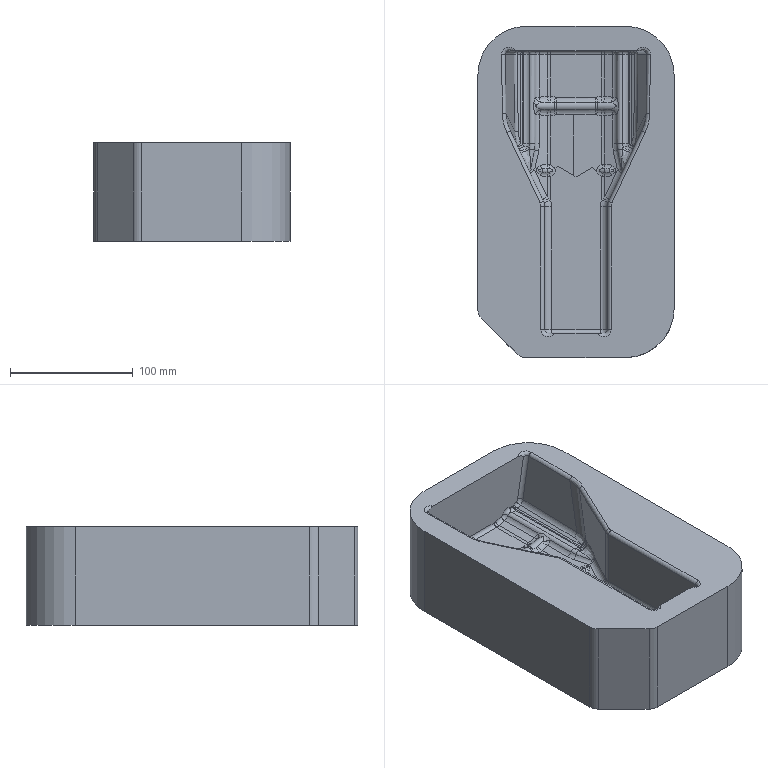NC program | NX | posted with a generic post | part box 160 x 270 x 80 mm
Lines 11488 to 12477 of 159324:
(ZLEVEL_PROFILE , TOOL : D16R0.8)
N22974 M6
N22976 G54
N22978 G17 G0 G90 X-41.264 Y99.089 S2000 M3
N22980 G43 Z10. H0
N22982 Z2.801
N22984 G94 G1 Z-0.199 F2000.
N22986 G3 X-49.234 Y107.089 R8.
N22988 G2 X-51.725 Y107.343 R12.794
N22990 G1 X-51.154 Y64.218
N22992 G3 X-48.351 Y52.165 R29.228
N22994 G1 X-21.353 Y-5.208
N22996 G2 X-19.849 Y-11.942 R15.824
N22998 G1 Y-107.329
N23000 G2 X-17.058 Y-107.089 R12.418
N23002 G1 X-17.202 Y-106.964 Z-0.399
N23004 G3 X-19.464 Y-107.098 R15.796
N23006 G1 Y-11.942
N23008 G3 X-21.005 Y-5.045 R16.209
N23010 G1 X-48.003 Y52.329
N23012 G2 X-50.77 Y64.256 R28.919
N23014 G1 X-51.337 Y107.111
N23016 G3 X-49.234 Y106.964 R14.071
N23018 G1 X-49.605 Y106.897 Z-0.598
N23020 X-51.031 Y106.963
N23022 X-50.465 Y64.227
N23024 G3 X-47.701 Y52.404 R28.679
N23026 G1 X-20.735 Y-4.902
N23028 G2 X-19.16 Y-11.942 R16.513
N23030 G1 Y-106.97
N23032 X-17.59 Y-106.898
N23034 X-17.299 Y-106.897
N23036 X-17.569 Y-106.885 Z-0.698
N23038 X-17.84 Y-106.875 Z-0.798
N23040 X-18.906 Y-106.886
N23042 Y-11.942
N23044 G3 X-20.498 Y-4.811 R16.767
N23046 G1 X-47.465 Y52.498
N23048 G2 X-50.213 Y64.315 R28.655
N23050 G1 X-50.776 Y106.897
N23052 X-49.917 Y106.875
N23054 G2 X-42.126 Y98.875 R8.
N23056 G1 Z2.202
N23058 G0 Z10.
N23060 X8.831 Y-99.089
N23062 Z2.801
N23064 G1 Z-0.199
N23066 X8.838 Y-99.326
N23068 G3 X17.068 Y-107.089 R8.
N23070 G2 X19.849 Y-107.333 R11.98
N23072 G1 Y-11.942
N23074 G2 X21.355 Y-5.203 R15.824
N23076 G1 X48.351 Y52.165
N23078 G3 X51.154 Y64.218 R29.228
N23080 G1 X51.725 Y107.339
N23082 G2 X49.244 Y107.089 R12.65
N23084 G1 Y107.018 Z-0.299
N23086 Y106.964 Z-0.399
N23088 G3 X51.337 Y107.111 R14.232
N23090 G1 X50.77 Y64.223
N23092 G2 X48.003 Y52.329 R28.844
N23094 G1 X21.005 Y-5.044
N23096 G3 X19.464 Y-11.942 R16.209
N23098 G1 Y-107.095
N23100 G3 X17.361 Y-106.964 R16.476
N23102 G1 X17.647 Y-106.897 Z-0.598
N23104 X19.16 Y-106.962
N23106 Y-11.942
N23108 G2 X20.735 Y-4.902 R16.513
N23110 G1 X47.704 Y52.41
N23112 G3 X50.465 Y64.227 R28.664
N23114 G1 X51.031 Y106.97
N23116 X49.401 Y106.898
N23118 X49.244 Y106.897
N23120 X49.581 Y106.888 Z-0.698
N23122 X49.919 Y106.875 Z-0.798
N23124 X50.776 Y106.898
N23126 X50.213 Y64.327
N23128 G2 X47.469 Y52.507 R28.661
N23130 G1 X20.504 Y-4.799
N23132 G3 X18.906 Y-11.942 R16.767
N23134 G1 Y-106.889
N23136 X17.836 Y-106.875
N23138 G2 X9.938 Y-98.875 R8.
N23140 G1 Z2.202
N23142 G0 Z10.
N23144 X8. Y98.875
N23146 Z2.003
N23148 G1 Z-0.997
N23150 G3 X0. Y106.875 R8.
N23152 G1 X-50.559
N23154 X-49.996 Y64.264
N23156 G3 X-47.339 Y52.738 R27.939
N23158 G1 X-20.298 Y-4.729
N23160 G2 X-18.69 Y-11.942 R16.983
N23162 G1 Y-106.875
N23164 X18.69
N23166 Y-11.942
N23168 G2 X20.308 Y-4.707 R16.983
N23170 G1 X47.282 Y52.617
N23172 G3 X49.995 Y64.233 R28.176
N23174 G1 X50.559 Y106.875
N23176 X0.
N23178 Z-1.197
N23180 X50.372
N23182 X49.808 Y64.236
N23184 G2 X47.115 Y52.701 R27.978
N23186 G1 X20.138 Y-4.627
N23188 G3 X18.502 Y-11.942 R17.171
N23190 G1 Y-106.875
N23192 X-18.502
N23194 Y-11.942
N23196 G3 X-20.128 Y-4.649 R17.171
N23198 G1 X-47.132 Y52.739
N23200 G2 X-49.808 Y64.236 R27.882
N23202 G1 X-50.372 Y106.875
N23204 X0.
N23206 Z-1.396
N23208 X-50.208
N23210 X-49.645 Y64.242
N23212 G3 X-46.984 Y52.808 R27.729
N23214 G1 X-19.988 Y-4.563
N23216 G2 X-18.339 Y-11.942 R17.334
N23218 G1 Y-106.875
N23220 X18.339
N23222 Y-11.942
N23224 G2 X19.989 Y-4.559 R17.334
N23226 G1 X46.969 Y52.775
N23228 G3 X49.645 Y64.272 R27.397
N23230 G1 X50.208 Y106.875
N23232 X0.
N23234 Z-1.596
N23236 X50.065
N23238 X49.501 Y64.24
N23240 G2 X46.84 Y52.839 R27.11
N23242 G1 X19.862 Y-4.493
N23244 G3 X18.195 Y-11.942 R17.478
N23246 G1 Y-106.875
N23248 X-18.195
N23250 Y-11.942
N23252 G3 X-19.855 Y-4.508 R17.478
N23254 G1 X-46.84 Y52.838
N23256 G2 X-49.501 Y64.24 R27.655
N23258 G1 X-50.065 Y106.875
N23260 X0.
N23262 Z-1.795
N23264 X-49.939
N23266 X-49.376 Y64.283
N23268 G3 X-46.741 Y52.923 R27.331
N23270 G1 X-19.741 Y-4.456
N23272 G2 X-18.07 Y-11.942 R17.603
N23274 G1 Y-106.875
N23276 X18.07
N23278 Y-11.942
N23280 G2 X19.748 Y-4.441 R17.603
N23282 G1 X46.741 Y52.923
N23284 G3 X49.375 Y64.242 R27.192
N23286 G1 X49.939 Y106.875
N23288 X0.
N23290 Z-1.995
N23292 X49.829
N23294 X49.267 Y64.327
N23296 G2 X46.633 Y52.952 R27.37
N23298 G1 X19.648 Y-4.395
N23300 G3 X17.96 Y-11.942 R17.713
N23302 G1 Y-106.875
N23304 X-17.96
N23306 Y-11.942
N23308 G3 X-19.641 Y-4.41 R17.713
N23310 G1 X-46.629 Y52.942
N23312 G2 X-49.266 Y64.304 R27.361
N23314 G1 X-49.829 Y106.875
N23316 X0.
N23318 Z-2.194
N23320 X-49.734
N23322 X-49.17 Y64.244
N23324 G3 X-46.555 Y53.01 R27.444
N23326 G1 X-19.554 Y-4.37
N23328 G2 X-17.864 Y-11.942 R17.809
N23330 G1 Y-106.875
N23332 X17.864
N23334 Y-11.942
N23336 G2 X19.561 Y-4.355 R17.809
N23338 G1 X46.555 Y53.01
N23340 G3 X49.17 Y64.251 R27.431
N23342 G1 X49.734 Y106.875
N23344 X0.
N23346 Z-2.393
N23348 X49.652
N23350 X49.088 Y64.245
N23352 G2 X46.465 Y53.013 R27.246
N23354 G1 X19.486 Y-4.321
N23356 G3 X17.782 Y-11.942 R17.891
N23358 G1 Y-106.875
N23360 X-17.782
N23362 Y-11.942
N23364 G3 X-19.479 Y-4.336 R17.891
N23366 G1 X-46.393 Y52.859
N23368 G2 X-49.089 Y64.309 R27.048
N23370 G1 X-49.652 Y106.875
N23372 X0.
N23374 Z-2.593
N23376 X-49.582
N23378 X-49.018 Y64.246
N23380 G3 X-46.405 Y53.049 R27.003
N23382 G1 X-19.416 Y-4.306
N23384 G2 X-17.712 Y-11.942 R17.961
N23386 G1 Y-106.875
N23388 X17.712
N23390 Y-11.942
N23392 G2 X19.422 Y-4.292 R17.961
N23394 G1 X46.417 Y53.074
N23396 G3 X49.019 Y64.303 R26.902
N23398 G1 X49.582 Y106.875
N23400 X0.
N23402 Z-2.792
N23404 X49.523
N23406 X48.96 Y64.247
N23408 X48.973 Y64.124
N23410 G2 X46.365 Y53.1 R27.521
N23412 G1 X19.369 Y-4.268
N23414 G3 X17.654 Y-11.942 R18.019
N23416 G1 Y-106.875
N23418 X-17.654
N23420 Y-11.942
N23422 G3 X-19.363 Y-4.282 R18.019
N23424 G1 X-46.365 Y53.1
N23426 G2 X-47.773 Y56.77 R25.554
N23428 X-48.96 Y64.247 R25.959
N23430 G1 X-49.523 Y106.875
N23432 X0.
N23434 Z-2.992
N23436 X-49.476
N23438 X-48.912 Y64.248
N23440 X-48.93 Y64.117
N23442 X-48.888 Y63.314
N23444 G3 X-46.335 Y53.147 R27.212
N23446 G1 X-19.32 Y-4.262
N23448 G2 X-17.607 Y-11.942 R18.066
N23450 G1 Y-106.875
N23452 X17.607
N23454 Y-11.942
N23456 G2 X19.327 Y-4.248 R18.066
N23458 G1 X46.322 Y53.12
N23460 G3 X48.922 Y64.069 R27.407
N23462 G1 X48.912 Y64.248
N23464 X49.476 Y106.875
N23466 X0.
N23468 Z-3.191
N23470 X49.439
N23472 X48.875 Y64.227
N23474 X48.878 Y64.109
N23476 G2 X46.289 Y53.136 R26.701
N23478 G1 X19.293 Y-4.233
N23480 G3 X17.57 Y-11.942 R18.103
N23482 G1 Y-106.875
N23484 X-17.57
N23486 Y-11.942
N23488 G3 X-19.287 Y-4.247 R18.103
N23490 G1 X-46.289 Y53.136
N23492 G2 X-48.88 Y64.591 R26.556
N23494 G1 X-49.439 Y106.875
N23496 X0.
N23498 Z-3.391
N23500 X-49.405
N23502 X-48.846 Y64.591
N23504 G3 X-46.212 Y53.033 R26.482
N23506 G1 X-19.263 Y-4.236
N23508 G2 X-17.544 Y-11.942 R18.129
N23510 G1 Y-106.875
N23512 X17.544
N23514 Y-11.942
N23516 G2 X19.27 Y-4.222 R18.129
N23518 G1 X46.266 Y53.147
N23520 G3 X48.841 Y64.202 R26.454
N23522 G1 X49.405 Y106.875
N23524 X0.
N23526 Z-3.59
N23528 X49.371
N23530 X48.806 Y64.165
N23532 G2 X46.251 Y53.153 R26.313
N23534 G1 X19.256 Y-4.216
N23536 G3 X17.529 Y-11.942 R18.144
N23538 G1 Y-106.875
N23540 X-17.529
N23542 Y-11.942
N23544 G3 X-19.249 Y-4.23 R18.144
N23546 G1 X-46.251 Y53.153
N23548 G2 X-48.806 Y64.166 R26.28
N23550 G1 X-49.371 Y106.875
N23552 X0.
N23554 Z-3.79
N23556 X-49.337
N23558 X-48.771 Y64.092
N23560 G3 X-46.309 Y53.293 R26.246
N23562 G1 X-46.209 Y53.075
N23564 X-39.382 Y38.567
N23566 X-19.254 Y-4.206
N23568 G2 X-17.524 Y-11.946 R18.178
N23570 G1 X-17.523 Y-106.875
N23572 X17.523
N23574 Y-106.807
N23576 X17.524 Y-11.943
N23578 G2 X19.253 Y-4.208 R18.166
N23580 G1 X40.363 Y40.652
N23582 X46.281 Y53.229
N23584 G3 X48.771 Y64.084 R26.343
N23586 G1 X49.337 Y106.875
N23588 X0.
N23590 Z-3.989
N23592 X49.303
N23594 X48.736 Y64.002
N23596 G2 X46.213 Y53.085 R26.467
N23598 G1 X19.251 Y-4.213
N23600 G3 X17.523 Y-11.942 R18.15
N23602 G1 Y-106.875
N23604 X-17.523
N23606 Y-11.942
N23608 G3 X-19.244 Y-4.228 R18.15
N23610 G1 X-46.213 Y53.085
N23612 G2 X-48.736 Y64.017 R26.384
N23614 G1 X-49.303 Y106.875
N23616 X0.
N23618 Z-4.189
N23620 X-49.269
N23622 X-48.701 Y63.943
N23624 G3 X-46.178 Y53.011 R26.501
N23626 G1 X-19.244 Y-4.228
N23628 G2 X-17.523 Y-11.942 R18.15
N23630 G1 Y-106.875
N23632 X17.523
N23634 Y-11.942
N23636 G2 X19.251 Y-4.213 R18.15
N23638 G1 X46.178 Y53.011
N23640 G3 X48.701 Y63.921 R26.451
N23642 G1 X49.269 Y106.875
N23644 X0.
N23646 Z-4.388
N23648 X49.235
N23650 X48.666 Y63.84
N23652 G2 X46.143 Y52.936 R26.435
N23654 G1 X19.251 Y-4.213
N23656 G3 X17.523 Y-11.942 R18.15
N23658 G1 Y-106.875
N23660 X-17.523
N23662 Y-11.942
N23664 G3 X-19.244 Y-4.228 R18.15
N23666 G1 X-46.143 Y52.936
N23668 G2 X-48.666 Y63.869 R26.502
N23670 G1 X-49.235 Y106.875
N23672 X0.
N23674 Z-4.587
N23676 X-49.201
N23678 X-48.631 Y63.794
N23680 G3 X-46.108 Y52.862 R26.502
N23682 G1 X-19.244 Y-4.228
N23684 G2 X-17.523 Y-11.942 R18.15
N23686 G1 Y-106.875
N23688 X17.523
N23690 Y-11.942
N23692 G2 X19.251 Y-4.213 R18.15
N23694 G1 X46.108 Y52.862
N23696 G3 X48.631 Y63.759 R26.42
N23698 G1 X49.201 Y106.875
N23700 X0.
N23702 Z-4.787
N23704 X49.167
N23706 X48.595 Y63.633
N23708 G2 X46.073 Y52.787 R26.301
N23710 G1 X19.251 Y-4.213
N23712 G3 X17.523 Y-11.942 R18.15
N23714 G1 Y-106.875
N23716 X-17.523
N23718 Y-11.942
N23720 G3 X-19.244 Y-4.228 R18.15
N23722 G1 X-46.073 Y52.787
N23724 G2 X-48.596 Y63.72 R26.502
N23726 G1 X-49.167 Y106.875
N23728 X0.
N23730 Z-4.986
N23732 X-49.133
N23734 X-48.561 Y63.614
N23736 G3 X-46.038 Y52.713 R26.428
N23738 G1 X-19.244 Y-4.228
N23740 G2 X-17.523 Y-11.942 R18.15
N23742 G1 Y-106.875
N23744 X17.523
N23746 Y-11.942
N23748 G2 X19.251 Y-4.213 R18.15
N23750 G1 X46.038 Y52.713
N23752 G3 X48.561 Y63.614 R26.428
N23754 G1 X49.133 Y106.875
N23756 X0.
N23758 Z-5.186
N23760 X49.099
N23762 X48.527 Y63.614
N23764 G2 X46.003 Y52.638 R26.6
N23766 G1 X19.251 Y-4.213
N23768 G3 X17.523 Y-11.942 R18.15
N23770 G1 Y-106.875
N23772 X-17.523
N23774 Y-11.942
N23776 G3 X-19.244 Y-4.228 R18.15
N23778 G1 X-46.003 Y52.638
N23780 G2 X-48.527 Y63.614 R26.6
N23782 G1 X-49.099 Y106.875
N23784 X0.
N23786 Z-5.385
N23788 X-49.065
N23790 X-48.493 Y63.614
N23792 G3 X-45.968 Y52.564 R26.772
N23794 G1 X-19.244 Y-4.228
N23796 G2 X-17.523 Y-11.942 R18.15
N23798 G1 Y-106.875
N23800 X17.523
N23802 Y-11.942
N23804 G2 X19.251 Y-4.213 R18.15
N23806 G1 X45.968 Y52.564
N23808 G3 X48.493 Y63.614 R26.772
N23810 G1 X49.065 Y106.875
N23812 X0.
N23814 Z-5.585
N23816 X49.031
N23818 X48.459 Y63.614
N23820 G2 X45.933 Y52.489 R26.944
N23822 G1 X19.251 Y-4.213
N23824 G3 X17.523 Y-11.942 R18.15
N23826 G1 Y-106.875
N23828 X-17.523
N23830 Y-11.942
N23832 G3 X-19.244 Y-4.228 R18.15
N23834 G1 X-45.933 Y52.489
N23836 G2 X-48.459 Y63.614 R26.944
N23838 G1 X-49.031 Y106.875
N23840 X0.
N23842 Z-5.784
N23844 X-48.997
N23846 X-48.425 Y63.614
N23848 G3 X-45.898 Y52.415 R27.116
N23850 G1 X-19.244 Y-4.228
N23852 G2 X-17.523 Y-11.942 R18.15
N23854 G1 Y-106.875
N23856 X17.523
N23858 Y-11.942
N23860 G2 X19.251 Y-4.213 R18.15
N23862 G1 X45.898 Y52.415
N23864 G3 X48.425 Y63.614 R27.116
N23866 G1 X48.997 Y106.875
N23868 X0.
N23870 Z-5.984
N23872 X48.963
N23874 X48.391 Y63.614
N23876 G2 X45.863 Y52.341 R26.789
N23878 G1 X19.251 Y-4.213
N23880 G3 X17.523 Y-11.942 R18.15
N23882 G1 Y-106.875
N23884 X-17.523
N23886 Y-11.942
N23888 G3 X-19.244 Y-4.228 R18.15
N23890 G1 X-45.863 Y52.341
N23892 G2 X-48.391 Y63.614 R26.749
N23894 G1 X-48.963 Y106.875
N23896 X0.
N23898 Z-6.183
N23900 X-48.929
N23902 X-48.357 Y63.614
N23904 G3 X-45.828 Y52.266 R26.857
N23906 G1 X-19.244 Y-4.228
N23908 G2 X-17.523 Y-11.942 R18.15
N23910 G1 Y-106.875
N23912 X17.523
N23914 Y-11.942
N23916 G2 X19.251 Y-4.213 R18.15
N23918 G1 X45.828 Y52.266
N23920 G3 X48.357 Y63.614 R26.874
N23922 G1 X48.929 Y106.875
N23924 X0.
N23926 Z-6.383
N23928 X48.895
N23930 X48.322 Y63.614
N23932 G2 X45.793 Y52.192 R26.951
N23934 G1 X19.251 Y-4.213
N23936 G3 X17.523 Y-11.942 R18.15
N23938 G1 Y-106.875
N23940 X-17.523
N23942 Y-11.942
N23944 G3 X-19.244 Y-4.228 R18.15
N23946 G1 X-45.793 Y52.192
N23948 G2 X-48.322 Y63.614 R27.147
N23950 G1 X-48.895 Y106.875
N23952 X0.
N23954 Z-6.582
N23956 X-48.861
N23958 X-48.281 Y63.062
N23960 G3 X-46.121 Y52.957 R26.344
N23962 G1 X-45.758 Y52.117
N23964 X-19.244 Y-4.228
N23966 G2 X-17.523 Y-11.942 R18.15
N23968 G1 Y-106.875
N23970 X17.523
N23972 Y-11.942
N23974 G2 X19.251 Y-4.213 R18.15
N23976 G1 X45.758 Y52.117
N23978 G3 X48.28 Y62.98 R27.072
N23980 G1 X48.288 Y63.614
N23982 X48.861 Y106.875
N23984 X0.
N23986 Z-6.781
N23988 X48.827
N23990 X48.245 Y62.894
N23992 G2 X47.418 Y56.77 R25.606
N23994 X45.723 Y52.043 R28.172
N23996 G1 X19.251 Y-4.213
N23998 G3 X17.523 Y-11.942 R18.15
N24000 G1 Y-106.875
N24002 X-17.523
N24004 Y-11.942
N24006 G3 X-19.244 Y-4.228 R18.15
N24008 G1 X-45.723 Y52.043
N24010 X-45.757 Y52.118
N24012 X-46.114 Y52.95
N24014 G2 X-48.246 Y62.989 R26.347
N24016 G1 X-48.827 Y106.875
N24018 X0.
N24020 Z-6.981
N24022 X-48.793
N24024 X-48.22 Y63.614
N24026 X-48.21 Y62.838
N24028 G3 X-45.917 Y52.497 R26.474
N24030 G1 X-45.884 Y52.427
N24032 X-45.722 Y52.043
N24034 X-45.688 Y51.968
N24036 X-19.244 Y-4.228
N24038 G2 X-17.523 Y-11.942 R18.15
N24040 G1 Y-106.875
N24042 X17.523
N24044 Y-11.942
N24046 G2 X19.251 Y-4.213 R18.15
N24048 G1 X45.688 Y51.968
N24050 G3 X47.294 Y56.34 R29.049
N24052 X48.213 Y63.04 R27.539
N24054 G1 X48.793 Y106.875
N24056 X0.
N24058 Z-7.18
N24060 X48.758
N24062 X48.178 Y62.96
N24064 G2 X47.294 Y56.403 R27.458
N24066 X45.653 Y51.894 R29.015
N24068 G1 X19.251 Y-4.213
N24070 G3 X17.523 Y-11.942 R18.15
N24072 G1 Y-106.875
N24074 X-17.523
N24076 Y-11.942
N24078 G3 X-19.244 Y-4.228 R18.15
N24080 G1 X-45.653 Y51.894
N24082 X-45.897 Y52.444
N24084 G2 X-48.177 Y62.876 R26.62
N24086 G1 X-48.758 Y106.875
N24088 X0.
N24090 Z-7.38
N24092 X-48.724
N24094 X-48.152 Y63.614
N24096 X-48.138 Y62.636
N24098 G3 X-46.127 Y52.982 R26.727
N24100 G1 X-46.072 Y52.859
N24102 X-45.618 Y51.819
N24104 X-19.244 Y-4.228
N24106 G2 X-17.523 Y-11.942 R18.15
N24108 G1 Y-106.875
N24110 X17.523
N24112 Y-11.942
N24114 G2 X19.251 Y-4.213 R18.15
N24116 G1 X45.618 Y51.819
N24118 G3 X47.294 Y56.466 R28.921
N24120 X48.143 Y62.882 R27.408
N24122 G1 X48.724 Y106.875
N24124 X0.
N24126 Z-7.579
N24128 X48.69
N24130 X48.105 Y62.636
N24132 G2 X47.294 Y56.529 R27.572
N24134 X45.583 Y51.745 R28.794
N24136 G1 X19.251 Y-4.213
N24138 G3 X17.523 Y-11.942 R18.15
N24140 G1 Y-106.875
N24142 X-17.523
N24144 Y-11.942
N24146 G3 X-19.244 Y-4.228 R18.15
N24148 G1 X-45.583 Y51.745
N24150 X-45.908 Y52.5
N24152 G2 X-48.105 Y62.636 R26.345
N24154 G1 X-48.69 Y106.875
N24156 X0.
N24158 Z-7.779
N24160 X-48.656
N24162 X-48.071 Y62.627
N24164 G3 X-45.887 Y52.453 R26.422
N24166 G1 X-45.548 Y51.671
N24168 X-19.244 Y-4.228
N24170 G2 X-17.523 Y-11.942 R18.15
N24172 G1 Y-106.875
N24174 X17.523
N24176 Y-11.942
N24178 G2 X19.251 Y-4.213 R18.15
N24180 G1 X45.548 Y51.671
N24182 G3 X47.294 Y56.592 R28.653
N24184 X48.071 Y62.636 R27.643
N24186 G1 X48.656 Y106.875
N24188 X0.
N24190 Z-7.978
N24192 X48.622
N24194 X48.037 Y62.636
N24196 G2 X47.294 Y56.655 R27.819
N24198 X45.513 Y51.596 R28.509
N24200 G1 X19.251 Y-4.213
N24202 G3 X17.523 Y-11.942 R18.15
N24204 G1 Y-106.875
N24206 X-17.523
N24208 Y-11.942
N24210 G3 X-19.244 Y-4.228 R18.15
N24212 G1 X-45.513 Y51.596
N24214 X-45.71 Y52.048
N24216 G2 X-48.037 Y62.636 R26.52
N24218 G1 X-48.622 Y106.875
N24220 X0.
N24222 Z-8.178
N24224 X-48.588
N24226 X-48.001 Y62.458
N24228 G3 X-45.843 Y52.367 R26.303
N24230 G1 X-45.477 Y51.522
N24232 X-19.244 Y-4.228
N24234 G2 X-17.523 Y-11.942 R18.15
N24236 G1 Y-106.875
N24238 X17.523
N24240 Y-11.942
N24242 G2 X19.251 Y-4.213 R18.15
N24244 G1 X45.477 Y51.522
N24246 G3 X47.307 Y56.77 R28.405
N24248 X48.003 Y62.636 R28.251
N24250 G1 X48.588 Y106.875
N24252 X0.
N24254 Z-8.377
N24256 X48.554
N24258 X47.969 Y62.636
N24260 G2 X47.294 Y56.787 R28.249
N24262 X45.442 Y51.447 R28.233
N24264 G1 X19.251 Y-4.213
N24266 G3 X17.523 Y-11.942 R18.15
N24268 G1 Y-106.875
N24270 X-17.523
N24272 Y-11.942
N24274 G3 X-19.244 Y-4.228 R18.15
N24276 G1 X-45.442 Y51.447
N24278 X-45.475 Y51.517
N24280 X-45.905 Y52.534
N24282 G2 X-47.965 Y62.363 R26.124
N24284 G1 X-48.554 Y106.875
N24286 X0.
N24288 Z-8.577
N24290 X-48.52
N24292 X-47.935 Y62.636
N24294 G3 X-45.407 Y51.373 R27.156
N24296 G1 X-19.244 Y-4.228
N24298 G2 X-17.523 Y-11.942 R18.15
N24300 G1 Y-106.875
N24302 X17.523
N24304 Y-11.942
N24306 G2 X19.251 Y-4.213 R18.15
N24308 G1 X45.407 Y51.373
N24310 G3 X47.935 Y62.636 R27.051
N24312 G1 X48.52 Y106.875
N24314 X0.
N24316 Z-8.776
N24318 X48.486
N24320 X47.895 Y62.191
N24322 G2 X47.736 Y59.703 R24.655
N24324 X45.372 Y51.298 R27.443
N24326 G1 X19.251 Y-4.213
N24328 G3 X17.523 Y-11.942 R18.15
N24330 G1 Y-106.875
N24332 X-17.523
N24334 Y-11.942
N24336 G3 X-19.244 Y-4.228 R18.15
N24338 G1 X-45.372 Y51.298
N24340 X-45.568 Y51.751
N24342 G2 X-47.901 Y62.636 R26.549
N24344 G1 X-48.486 Y106.875
N24346 X0.
N24348 Z-8.975
N24350 X-48.452
N24352 X-47.861 Y62.186
N24354 G3 X-45.682 Y52.02 R26.443
N24356 G1 X-45.337 Y51.224
N24358 X-19.244 Y-4.228
N24360 G2 X-17.523 Y-11.942 R18.15
N24362 G1 Y-106.875
N24364 X17.523
N24366 Y-11.942
N24368 G2 X19.251 Y-4.213 R18.15
N24370 G1 X45.337 Y51.224
N24372 G3 X47.294 Y57.061 R28.268
N24374 X47.867 Y62.636 R28.066
N24376 G1 X48.452 Y106.875
N24378 X0.
N24380 Z-9.175
N24382 X48.418
N24384 X47.833 Y62.636
N24386 G2 X46.977 Y55.792 R27.54
N24388 X45.302 Y51.149 R28.898
N24390 G1 X19.251 Y-4.213
N24392 G3 X17.523 Y-11.942 R18.15
N24394 G1 Y-106.875
N24396 X-17.523
N24398 Y-11.942
N24400 G3 X-19.244 Y-4.228 R18.15
N24402 G1 X-45.302 Y51.149
N24404 X-45.435 Y51.45
N24406 X-45.462 Y51.522
N24408 X-45.785 Y52.288
N24410 G2 X-47.825 Y62.069 R26.119
N24412 G1 X-48.418 Y106.875
N24414 X0.
N24416 Z-9.374
N24418 X-48.384
N24420 X-47.791 Y62.045
N24422 G3 X-45.591 Y51.818 R26.498
N24424 G1 X-45.267 Y51.075
N24426 X-19.244 Y-4.228
N24428 G2 X-17.523 Y-11.942 R18.15
N24430 G1 Y-106.875
N24432 X17.523
N24434 Y-11.942
N24436 G2 X19.251 Y-4.213 R18.15
N24438 G1 X45.267 Y51.075
N24440 G3 X46.96 Y55.792 R28.902
N24442 X47.789 Y61.929 R27.436
N24444 G1 X47.799 Y62.636
N24446 X48.384 Y106.875
N24448 X0.
N24450 Z-9.574
N24452 X48.35
N24454 X47.765 Y62.636
N24456 X47.754 Y61.854
N24458 G2 X46.944 Y55.792 R27.536
N24460 X45.232 Y51. R28.815
N24462 G1 X19.251 Y-4.213
N24464 G3 X17.523 Y-11.942 R18.15
N24466 G1 Y-106.875
N24468 X-17.523
N24470 Y-11.942
N24472 G3 X-19.244 Y-4.228 R18.15
N24474 G1 X-45.232 Y51.
N24476 X-45.59 Y51.829
N24478 G2 X-47.756 Y61.958 R26.409
N24480 G1 X-48.35 Y106.875
N24482 X0.
N24484 Z-9.773
N24486 X-48.316
N24488 X-47.731 Y62.636
N24490 X-47.719 Y61.787
N24492 G3 X-45.363 Y51.302 R26.896
N24494 G1 X-45.197 Y50.926
N24496 X-19.244 Y-4.228
N24498 G2 X-17.523 Y-11.942 R18.15
N24500 G1 Y-106.875
N24502 X17.523
N24504 Y-11.942
N24506 G2 X19.251 Y-4.213 R18.15
N24508 G1 X45.197 Y50.926
N24510 G3 X46.928 Y55.792 R28.662
N24512 X47.722 Y61.993 R27.434
N24514 G1 X48.316 Y106.875
N24516 X0.
N24518 Z-9.973
N24520 X48.282
N24522 X47.697 Y62.636
N24524 X47.684 Y61.703
N24526 X47.642 Y60.681
N24528 G2 X45.162 Y50.852 R27.387
N24530 G1 X19.251 Y-4.213
N24532 G3 X17.523 Y-11.942 R18.15
N24534 G1 Y-106.875
N24536 X-17.523
N24538 Y-11.942
N24540 G3 X-19.244 Y-4.228 R18.15
N24542 G1 X-45.162 Y50.852
N24544 X-45.48 Y51.581
N24546 G2 X-47.686 Y61.817 R26.485
N24548 G1 X-48.282 Y106.875
N24550 X0.
N24552 Z-10.172
N24554 X-48.248
N24556 X-47.65 Y61.658
N24558 G3 X-45.334 Y51.245 R26.876
N24560 G1 X-45.291 Y51.154
N24562 X-45.127 Y50.777
N24564 X-19.244 Y-4.228
N24566 G2 X-17.523 Y-11.942 R18.15
N24568 G1 Y-106.875
N24570 X17.523
N24572 Y-11.942
N24574 G2 X19.251 Y-4.213 R18.15
N24576 G1 X45.127 Y50.777
N24578 G3 X47.65 Y61.658 R27.272
N24580 G1 X48.248 Y106.875
N24582 X0.
N24584 Z-10.372
N24586 X48.214
N24588 X47.616 Y61.658
N24590 G2 X45.092 Y50.703 R27.197
N24592 G1 X19.251 Y-4.213
N24594 G3 X17.523 Y-11.942 R18.15
N24596 G1 Y-106.875
N24598 X-17.523
N24600 Y-11.942
N24602 G3 X-19.244 Y-4.228 R18.15
N24604 G1 X-45.092 Y50.703
N24606 X-45.288 Y51.156
N24608 G2 X-47.616 Y61.658 R26.539
N24610 G1 X-48.214 Y106.875
N24612 X0.
N24614 Z-10.571
N24616 X-48.18
N24618 X-47.582 Y61.658
N24620 G3 X-45.175 Y50.903 R26.587
N24622 G1 X-45.157 Y50.854
N24624 X-45.057 Y50.628
N24626 X-19.244 Y-4.228
N24628 G2 X-17.523 Y-11.942 R18.15
N24630 G1 Y-106.875
N24632 X17.523
N24634 Y-11.942
N24636 G2 X19.251 Y-4.213 R18.15
N24638 G1 X45.057 Y50.628
N24640 G3 X47.582 Y61.658 R27.216
N24642 G1 X48.18 Y106.875
N24644 X0.
N24646 Z-10.771
N24648 X48.146
N24650 X47.546 Y61.532
N24652 G2 X47.356 Y58.725 R25.877
N24654 X45.022 Y50.554 R27.311
N24656 G1 X19.251 Y-4.213
N24658 G3 X17.523 Y-11.942 R18.15
N24660 G1 Y-106.875
N24662 X-17.523
N24664 Y-11.942
N24666 G3 X-19.244 Y-4.228 R18.15
N24668 G1 X-45.022 Y50.554
N24670 X-45.154 Y50.855
N24672 X-45.172 Y50.903
N24674 G2 X-47.548 Y61.658 R26.521
N24676 G1 X-48.146 Y106.875
N24678 X0.
N24680 Z-10.97
N24682 X-48.112
N24684 X-47.513 Y61.658
N24686 G3 X-45.184 Y50.932 R26.548
N24688 G1 X-44.987 Y50.479
N24690 X-19.244 Y-4.228
N24692 G2 X-17.523 Y-11.942 R18.15
N24694 G1 Y-106.875
N24696 X17.523
N24698 Y-11.942
N24700 G2 X19.251 Y-4.213 R18.15
N24702 G1 X44.987 Y50.479
N24704 G3 X47.302 Y58.477 R27.335
N24706 X47.51 Y61.399 R25.345
N24708 G1 X48.112 Y106.875
N24710 X0.
N24712 Z-11.169
N24714 X48.077
N24716 X47.475 Y61.326
N24718 G2 X47.315 Y58.8 R25.241
N24720 X44.952 Y50.405 R27.233
N24722 G1 X19.251 Y-4.213
N24724 G3 X17.523 Y-11.942 R18.15
N24726 G1 Y-106.875
N24728 X-17.523
N24730 Y-11.942
N24732 G3 X-19.244 Y-4.228 R18.15
N24734 G1 X-44.952 Y50.405
N24736 X-45.148 Y50.857
N24738 G2 X-47.479 Y61.658 R26.508
N24740 G1 X-48.077 Y106.875
N24742 X0.
N24744 Z-11.369
N24746 X-48.043
N24748 X-47.44 Y61.27
N24750 G3 X-45.27 Y51.145 R26.331
N24752 G1 X-44.917 Y50.33
N24754 X-19.244 Y-4.228
N24756 G2 X-17.523 Y-11.942 R18.15
N24758 G1 Y-106.875
N24760 X17.523
N24762 Y-11.942
N24764 G2 X19.251 Y-4.213 R18.15
N24766 G1 X44.917 Y50.33
N24768 G3 X47.445 Y61.658 R27.041
N24770 G1 X48.043 Y106.875
N24772 X0.
N24774 Z-11.568
N24776 X48.009
N24778 X47.411 Y61.658
N24780 G2 X44.882 Y50.256 R26.959
N24782 G1 X19.251 Y-4.213
N24784 G3 X17.523 Y-11.942 R18.15
N24786 G1 Y-106.875
N24788 X-17.523
N24790 Y-11.942
N24792 G3 X-19.244 Y-4.228 R18.15
N24794 G1 X-44.882 Y50.256
N24796 G2 X-47.411 Y61.658 R27.22
N24798 G1 X-48.009 Y106.875
N24800 X0.
N24802 Z-11.768
N24804 X-47.975
N24806 X-47.377 Y61.658
N24808 G3 X-44.847 Y50.182 R27.12
N24810 G1 X-19.244 Y-4.228
N24812 G2 X-17.523 Y-11.942 R18.15
N24814 G1 Y-106.875
N24816 X17.523
N24818 Y-11.942
N24820 G2 X19.251 Y-4.213 R18.15
N24822 G1 X44.847 Y50.181
N24824 G3 X47.369 Y61.026 R26.971
N24826 G1 X47.377 Y61.658
N24828 X47.975 Y106.875
N24830 X0.
N24832 Z-11.967
N24834 X47.941
N24836 X47.334 Y60.951
N24838 G2 X44.812 Y50.107 R27.123
N24840 G1 X19.251 Y-4.213
N24842 G3 X17.523 Y-11.942 R18.15
N24844 G1 Y-106.875
N24846 X-17.523
N24848 Y-11.942
N24850 G3 X-19.244 Y-4.228 R18.15
N24852 G1 X-44.812 Y50.107
N24854 G2 X-47.334 Y60.965 R26.961
N24856 G1 X-47.343 Y61.658
N24858 X-47.941 Y106.875
N24860 X0.
N24862 Z-12.167
N24864 X-47.907
N24866 X-47.309 Y61.658
N24868 X-47.299 Y60.891
N24870 G3 X-44.777 Y50.033 R27.011
N24872 G1 X-19.244 Y-4.228
N24874 G2 X-17.523 Y-11.942 R18.15
N24876 G1 Y-106.875
N24878 X17.523
N24880 Y-11.942
N24882 G2 X19.251 Y-4.213 R18.15
N24884 G1 X44.777 Y50.033
N24886 G3 X47.299 Y60.877 R27.204
N24888 G1 X47.907 Y106.875
N24890 X0.
N24892 Z-12.366
N24894 X47.873
N24896 X47.264 Y60.802
N24898 G2 X44.742 Y49.958 R27.232
N24900 G1 X19.251 Y-4.213
N24902 G3 X17.523 Y-11.942 R18.15
N24904 G1 Y-106.875
N24906 X-17.523
N24908 Y-11.942
N24910 G3 X-19.244 Y-4.228 R18.15
N24912 G1 X-44.742 Y49.958
N24914 G2 X-47.264 Y60.817 R27.207
N24916 G1 X-47.275 Y61.658
N24918 X-47.873 Y106.875
N24920 X0.
N24922 Z-12.566
N24924 X-47.839
N24926 X-47.241 Y61.658
N24928 X-47.229 Y60.743
N24930 G3 X-44.726 Y49.926 R27.275
N24932 G1 X-44.707 Y49.884
N24934 X-19.244 Y-4.228
N24936 G2 X-17.523 Y-11.942 R18.15
N24938 G1 Y-106.875
N24940 X17.523
N24942 Y-11.942
N24944 G2 X19.251 Y-4.213 R18.15
N24946 G1 X44.707 Y49.884